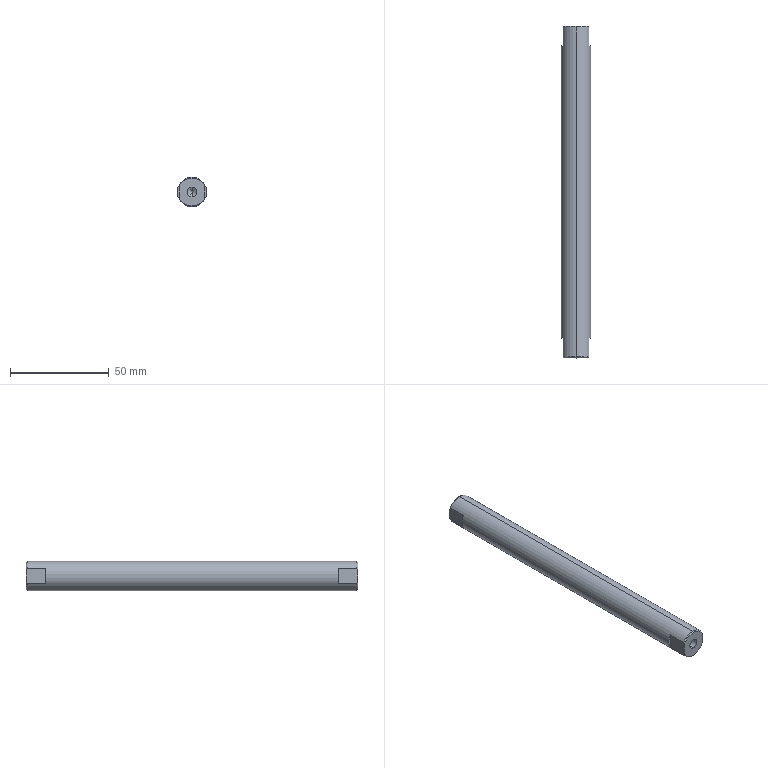Part | SolidWorks | features Chamfer 1, Extrusion 1, HoleWzd 1, ICE 1, MirrorPattern 1 | 1 solid | 26 faces | box 15 x 168 x 15 mm | volume 28790 mm3 | cone 10 | plane 10 | cylinder 6 | commonest cylinder face diameters 5 x4 15 x2
STEP:
#1=CARTESIAN_POINT('',(0.,-67.,2.5));
#2=VERTEX_POINT('',#1);
#3=CARTESIAN_POINT('',(0.,-67.,-2.5));
#4=VERTEX_POINT('',#3);
#5=CARTESIAN_POINT('',(0.,-67.,0.));
#6=DIRECTION('',(0.,-1.,0.));
#7=DIRECTION('',(0.,0.,-1.));
#8=AXIS2_PLACEMENT_3D('',#5,#6,#7);
#9=CIRCLE('',#8,2.5);
#10=EDGE_CURVE('',#2,#4,#9,.T.);
#11=ORIENTED_EDGE('',*,*,#10,.F.);
#12=CARTESIAN_POINT('',(0.,-84.,2.5));
#13=VERTEX_POINT('',#12);
#14=CARTESIAN_POINT('',(0.,-84.,2.5));
#15=DIRECTION('',(0.,-1.,0.));
#16=VECTOR('',#15,1000.);
#17=LINE('',#14,#16);
#18=EDGE_CURVE('',#2,#13,#17,.T.);
#19=ORIENTED_EDGE('',*,*,#18,.T.);
#20=CARTESIAN_POINT('',(0.,-84.,-2.5));
#21=VERTEX_POINT('',#20);
#22=CARTESIAN_POINT('',(0.,-84.,0.));
#23=DIRECTION('',(0.,-1.,0.));
#24=DIRECTION('',(0.,0.,-1.));
#25=AXIS2_PLACEMENT_3D('',#22,#23,#24);
#26=CIRCLE('',#25,2.5);
#27=EDGE_CURVE('',#13,#21,#26,.T.);
#28=ORIENTED_EDGE('',*,*,#27,.T.);
#29=CARTESIAN_POINT('',(0.,-84.,-2.5));
#30=DIRECTION('',(0.,-1.,0.));
#31=VECTOR('',#30,1000.);
#32=LINE('',#29,#31);
#33=EDGE_CURVE('',#4,#21,#32,.T.);
#34=ORIENTED_EDGE('',*,*,#33,.F.);
#35=EDGE_LOOP('',(#11,#19,#28,#34));
#36=FACE_OUTER_BOUND('',#35,.T.);
#37=CARTESIAN_POINT('',(0.,-84.,0.));
#38=DIRECTION('',(0.,-1.,0.));
#39=DIRECTION('',(0.,0.,-1.));
#40=AXIS2_PLACEMENT_3D('',#37,#38,#39);
#41=CYLINDRICAL_SURFACE('',#40,2.5);
#42=ADVANCED_FACE('',(#36),#41,.F.);
#43=CARTESIAN_POINT('',(0.,-65.498,0.));
#44=VERTEX_POINT('',#43);
#45=CARTESIAN_POINT('',(0.,-67.,-2.5));
#46=DIRECTION('',(0.,-0.515,-0.8572));
#47=VECTOR('',#46,1000.);
#48=LINE('',#45,#47);
#49=EDGE_CURVE('',#44,#4,#48,.T.);
#50=ORIENTED_EDGE('',*,*,#49,.F.);
#51=CARTESIAN_POINT('',(0.,-67.,2.5));
#52=DIRECTION('',(0.,-0.515,0.8572));
#53=VECTOR('',#52,1000.);
#54=LINE('',#51,#53);
#55=EDGE_CURVE('',#44,#2,#54,.T.);
#56=ORIENTED_EDGE('',*,*,#55,.T.);
#57=ORIENTED_EDGE('',*,*,#10,.T.);
#58=EDGE_LOOP('',(#50,#56,#57));
#59=FACE_OUTER_BOUND('',#58,.T.);
#60=CARTESIAN_POINT('',(0.,-67.,0.));
#61=DIRECTION('',(0.,-1.,0.));
#62=DIRECTION('',(0.,0.,-1.));
#63=AXIS2_PLACEMENT_3D('',#60,#61,#62);
#64=CONICAL_SURFACE('',#63,2.5,1.03);
#65=ADVANCED_FACE('',(#59),#64,.F.);
#66=CARTESIAN_POINT('',(0.,67.,-2.5));
#67=VERTEX_POINT('',#66);
#68=CARTESIAN_POINT('',(0.,67.,2.5));
#69=VERTEX_POINT('',#68);
#70=CARTESIAN_POINT('',(0.,67.,0.));
#71=DIRECTION('',(0.,1.,0.));
#72=DIRECTION('',(0.,0.,1.));
#73=AXIS2_PLACEMENT_3D('',#70,#71,#72);
#74=CIRCLE('',#73,2.5);
#75=EDGE_CURVE('',#67,#69,#74,.T.);
#76=ORIENTED_EDGE('',*,*,#75,.F.);
#77=CARTESIAN_POINT('',(0.,84.,-2.5));
#78=VERTEX_POINT('',#77);
#79=CARTESIAN_POINT('',(0.,84.,-2.5));
#80=DIRECTION('',(0.,1.,0.));
#81=VECTOR('',#80,1000.);
#82=LINE('',#79,#81);
#83=EDGE_CURVE('',#67,#78,#82,.T.);
#84=ORIENTED_EDGE('',*,*,#83,.T.);
#85=CARTESIAN_POINT('',(0.,84.,2.5));
#86=VERTEX_POINT('',#85);
#87=CARTESIAN_POINT('',(0.,84.,0.));
#88=DIRECTION('',(0.,1.,0.));
#89=DIRECTION('',(0.,0.,1.));
#90=AXIS2_PLACEMENT_3D('',#87,#88,#89);
#91=CIRCLE('',#90,2.5);
#92=EDGE_CURVE('',#78,#86,#91,.T.);
#93=ORIENTED_EDGE('',*,*,#92,.T.);
#94=CARTESIAN_POINT('',(0.,84.,2.5));
#95=DIRECTION('',(0.,1.,0.));
#96=VECTOR('',#95,1000.);
#97=LINE('',#94,#96);
#98=EDGE_CURVE('',#69,#86,#97,.T.);
#99=ORIENTED_EDGE('',*,*,#98,.F.);
#100=EDGE_LOOP('',(#76,#84,#93,#99));
#101=FACE_OUTER_BOUND('',#100,.T.);
#102=CARTESIAN_POINT('',(0.,84.,0.));
#103=DIRECTION('',(0.,1.,0.));
#104=DIRECTION('',(0.,0.,1.));
#105=AXIS2_PLACEMENT_3D('',#102,#103,#104);
#106=CYLINDRICAL_SURFACE('',#105,2.5);
#107=ADVANCED_FACE('',(#101),#106,.F.);
#108=CARTESIAN_POINT('',(0.,65.498,0.));
#109=VERTEX_POINT('',#108);
#110=CARTESIAN_POINT('',(0.,67.,2.5));
#111=DIRECTION('',(0.,0.515,0.8572));
#112=VECTOR('',#111,1000.);
#113=LINE('',#110,#112);
#114=EDGE_CURVE('',#109,#69,#113,.T.);
#115=ORIENTED_EDGE('',*,*,#114,.F.);
#116=CARTESIAN_POINT('',(0.,67.,-2.5));
#117=DIRECTION('',(0.,0.515,-0.8572));
#118=VECTOR('',#117,1000.);
#119=LINE('',#116,#118);
#120=EDGE_CURVE('',#109,#67,#119,.T.);
#121=ORIENTED_EDGE('',*,*,#120,.T.);
#122=ORIENTED_EDGE('',*,*,#75,.T.);
#123=EDGE_LOOP('',(#115,#121,#122));
#124=FACE_OUTER_BOUND('',#123,.T.);
#125=CARTESIAN_POINT('',(0.,67.,0.));
#126=DIRECTION('',(0.,1.,0.));
#127=DIRECTION('',(0.,0.,1.));
#128=AXIS2_PLACEMENT_3D('',#125,#126,#127);
#129=CONICAL_SURFACE('',#128,2.5,1.03);
#130=ADVANCED_FACE('',(#124),#129,.F.);
#131=CARTESIAN_POINT('',(0.,-84.,7.));
#132=VERTEX_POINT('',#131);
#133=CARTESIAN_POINT('',(-6.5,-84.,2.598));
#134=VERTEX_POINT('',#133);
#135=CARTESIAN_POINT('',(0.,-84.,0.));
#136=DIRECTION('',(0.,-1.,0.));
#137=DIRECTION('',(0.,0.,1.));
#138=AXIS2_PLACEMENT_3D('',#135,#136,#137);
#139=CIRCLE('',#138,7.);
#140=EDGE_CURVE('',#132,#134,#139,.T.);
#141=ORIENTED_EDGE('',*,*,#140,.F.);
#142=CARTESIAN_POINT('',(0.,-83.5,7.5));
#143=VERTEX_POINT('',#142);
#144=CARTESIAN_POINT('',(0.,-83.5,7.5));
#145=DIRECTION('',(0.,0.7071,0.7071));
#146=VECTOR('',#145,1000.);
#147=LINE('',#144,#146);
#148=EDGE_CURVE('',#132,#143,#147,.T.);
#149=ORIENTED_EDGE('',*,*,#148,.T.);
#150=CARTESIAN_POINT('',(-6.5,-83.5,3.742));
#151=VERTEX_POINT('',#150);
#152=CARTESIAN_POINT('',(0.,-83.5,0.));
#153=DIRECTION('',(0.,1.,0.));
#154=DIRECTION('',(0.,0.,1.));
#155=AXIS2_PLACEMENT_3D('',#152,#153,#154);
#156=CIRCLE('',#155,7.5);
#157=EDGE_CURVE('',#151,#143,#156,.T.);
#158=ORIENTED_EDGE('',*,*,#157,.F.);
#159=CARTESIAN_POINT('',(-6.5,-84.,2.598));
#160=CARTESIAN_POINT('',(-6.5,-83.854,2.991));
#161=CARTESIAN_POINT('',(-6.5,-83.685,3.371));
#162=CARTESIAN_POINT('',(-6.5,-83.5,3.742));
#163=B_SPLINE_CURVE_WITH_KNOTS('',3,(#159,#160,#161,#162),.UNSPECIFIED.,.F.,.F.,(4,4),(0.02116,0.02241),.UNSPECIFIED.);
#164=EDGE_CURVE('',#134,#151,#163,.T.);
#165=ORIENTED_EDGE('',*,*,#164,.F.);
#166=EDGE_LOOP('',(#141,#149,#158,#165));
#167=FACE_OUTER_BOUND('',#166,.T.);
#168=CARTESIAN_POINT('',(0.,-83.5,0.));
#169=DIRECTION('',(0.,1.,0.));
#170=DIRECTION('',(0.,0.,1.));
#171=AXIS2_PLACEMENT_3D('',#168,#169,#170);
#172=CONICAL_SURFACE('',#171,7.5,0.7854);
#173=ADVANCED_FACE('',(#167),#172,.T.);
#174=CARTESIAN_POINT('',(6.5,83.5,3.742));
#175=VERTEX_POINT('',#174);
#176=CARTESIAN_POINT('',(0.,83.5,7.5));
#177=VERTEX_POINT('',#176);
#178=CARTESIAN_POINT('',(0.,83.5,0.));
#179=DIRECTION('',(0.,-1.,0.));
#180=DIRECTION('',(0.,0.,1.));
#181=AXIS2_PLACEMENT_3D('',#178,#179,#180);
#182=CIRCLE('',#181,7.5);
#183=EDGE_CURVE('',#175,#177,#182,.T.);
#184=ORIENTED_EDGE('',*,*,#183,.T.);
#185=CARTESIAN_POINT('',(0.,84.,7.5));
#186=DIRECTION('',(0.,-1.,0.));
#187=VECTOR('',#186,1000.);
#188=LINE('',#185,#187);
#189=EDGE_CURVE('',#177,#143,#188,.T.);
#190=ORIENTED_EDGE('',*,*,#189,.T.);
#191=CARTESIAN_POINT('',(6.5,-83.5,3.742));
#192=VERTEX_POINT('',#191);
#193=CARTESIAN_POINT('',(0.,-83.5,0.));
#194=DIRECTION('',(0.,1.,0.));
#195=DIRECTION('',(0.,0.,1.));
#196=AXIS2_PLACEMENT_3D('',#193,#194,#195);
#197=CIRCLE('',#196,7.5);
#198=EDGE_CURVE('',#143,#192,#197,.T.);
#199=ORIENTED_EDGE('',*,*,#198,.T.);
#200=CARTESIAN_POINT('',(6.5,-74.,3.742));
#201=VERTEX_POINT('',#200);
#202=CARTESIAN_POINT('',(6.5,84.,3.742));
#203=DIRECTION('',(0.,1.,0.));
#204=VECTOR('',#203,1000.);
#205=LINE('',#202,#204);
#206=EDGE_CURVE('',#192,#201,#205,.T.);
#207=ORIENTED_EDGE('',*,*,#206,.T.);
#208=CARTESIAN_POINT('',(6.5,-74.,-3.742));
#209=VERTEX_POINT('',#208);
#210=CARTESIAN_POINT('',(0.,-74.,0.));
#211=DIRECTION('',(0.,1.,0.));
#212=DIRECTION('',(0.,0.,1.));
#213=AXIS2_PLACEMENT_3D('',#210,#211,#212);
#214=CIRCLE('',#213,7.5);
#215=EDGE_CURVE('',#201,#209,#214,.T.);
#216=ORIENTED_EDGE('',*,*,#215,.T.);
#217=CARTESIAN_POINT('',(6.5,-83.5,-3.742));
#218=VERTEX_POINT('',#217);
#219=CARTESIAN_POINT('',(6.5,84.,-3.742));
#220=DIRECTION('',(0.,-1.,0.));
#221=VECTOR('',#220,1000.);
#222=LINE('',#219,#221);
#223=EDGE_CURVE('',#209,#218,#222,.T.);
#224=ORIENTED_EDGE('',*,*,#223,.T.);
#225=CARTESIAN_POINT('',(0.,-83.5,-7.5));
#226=VERTEX_POINT('',#225);
#227=CARTESIAN_POINT('',(0.,-83.5,0.));
#228=DIRECTION('',(0.,1.,0.));
#229=DIRECTION('',(0.,0.,1.));
#230=AXIS2_PLACEMENT_3D('',#227,#228,#229);
#231=CIRCLE('',#230,7.5);
#232=EDGE_CURVE('',#218,#226,#231,.T.);
#233=ORIENTED_EDGE('',*,*,#232,.T.);
#234=CARTESIAN_POINT('',(0.,83.5,-7.5));
#235=VERTEX_POINT('',#234);
#236=CARTESIAN_POINT('',(0.,84.,-7.5));
#237=DIRECTION('',(0.,-1.,0.));
#238=VECTOR('',#237,1000.);
#239=LINE('',#236,#238);
#240=EDGE_CURVE('',#235,#226,#239,.T.);
#241=ORIENTED_EDGE('',*,*,#240,.F.);
#242=CARTESIAN_POINT('',(6.5,83.5,-3.742));
#243=VERTEX_POINT('',#242);
#244=CARTESIAN_POINT('',(0.,83.5,0.));
#245=DIRECTION('',(0.,-1.,0.));
#246=DIRECTION('',(0.,0.,1.));
#247=AXIS2_PLACEMENT_3D('',#244,#245,#246);
#248=CIRCLE('',#247,7.5);
#249=EDGE_CURVE('',#235,#243,#248,.T.);
#250=ORIENTED_EDGE('',*,*,#249,.T.);
#251=CARTESIAN_POINT('',(6.5,74.,-3.742));
#252=VERTEX_POINT('',#251);
#253=CARTESIAN_POINT('',(6.5,84.,-3.742));
#254=DIRECTION('',(0.,-1.,0.));
#255=VECTOR('',#254,1000.);
#256=LINE('',#253,#255);
#257=EDGE_CURVE('',#243,#252,#256,.T.);
#258=ORIENTED_EDGE('',*,*,#257,.T.);
#259=CARTESIAN_POINT('',(6.5,74.,3.742));
#260=VERTEX_POINT('',#259);
#261=CARTESIAN_POINT('',(0.,74.,0.));
#262=DIRECTION('',(0.,-1.,0.));
#263=DIRECTION('',(0.,0.,-1.));
#264=AXIS2_PLACEMENT_3D('',#261,#262,#263);
#265=CIRCLE('',#264,7.5);
#266=EDGE_CURVE('',#252,#260,#265,.T.);
#267=ORIENTED_EDGE('',*,*,#266,.T.);
#268=CARTESIAN_POINT('',(6.5,84.,3.742));
#269=DIRECTION('',(0.,1.,0.));
#270=VECTOR('',#269,1000.);
#271=LINE('',#268,#270);
#272=EDGE_CURVE('',#260,#175,#271,.T.);
#273=ORIENTED_EDGE('',*,*,#272,.T.);
#274=EDGE_LOOP('',(#184,#190,#199,#207,#216,#224,#233,#241,#250,#258,#267,#273));
#275=FACE_OUTER_BOUND('',#274,.T.);
#276=CARTESIAN_POINT('',(0.,84.,0.));
#277=DIRECTION('',(0.,-1.,0.));
#278=DIRECTION('',(0.,0.,-1.));
#279=AXIS2_PLACEMENT_3D('',#276,#277,#278);
#280=CYLINDRICAL_SURFACE('',#279,7.5);
#281=ADVANCED_FACE('',(#275),#280,.T.);
#282=CARTESIAN_POINT('',(0.,84.,-7.));
#283=VERTEX_POINT('',#282);
#284=CARTESIAN_POINT('',(-6.5,84.,-2.598));
#285=VERTEX_POINT('',#284);
#286=CARTESIAN_POINT('',(0.,84.,0.));
#287=DIRECTION('',(0.,1.,0.));
#288=DIRECTION('',(0.,0.,1.));
#289=AXIS2_PLACEMENT_3D('',#286,#287,#288);
#290=CIRCLE('',#289,7.);
#291=EDGE_CURVE('',#283,#285,#290,.T.);
#292=ORIENTED_EDGE('',*,*,#291,.F.);
#293=CARTESIAN_POINT('',(0.,84.,-7.));
#294=DIRECTION('',(0.,-0.7071,-0.7071));
#295=VECTOR('',#294,1000.);
#296=LINE('',#293,#295);
#297=EDGE_CURVE('',#283,#235,#296,.T.);
#298=ORIENTED_EDGE('',*,*,#297,.T.);
#299=CARTESIAN_POINT('',(-6.5,83.5,-3.742));
#300=VERTEX_POINT('',#299);
#301=CARTESIAN_POINT('',(0.,83.5,0.));
#302=DIRECTION('',(0.,-1.,0.));
#303=DIRECTION('',(0.,0.,1.));
#304=AXIS2_PLACEMENT_3D('',#301,#302,#303);
#305=CIRCLE('',#304,7.5);
#306=EDGE_CURVE('',#300,#235,#305,.T.);
#307=ORIENTED_EDGE('',*,*,#306,.F.);
#308=CARTESIAN_POINT('',(-6.5,84.,-2.598));
#309=CARTESIAN_POINT('',(-6.5,83.854,-2.991));
#310=CARTESIAN_POINT('',(-6.5,83.685,-3.371));
#311=CARTESIAN_POINT('',(-6.5,83.5,-3.742));
#312=B_SPLINE_CURVE_WITH_KNOTS('',3,(#308,#309,#310,#311),.UNSPECIFIED.,.F.,.F.,(4,4),(0.02116,0.02241),.UNSPECIFIED.);
#313=EDGE_CURVE('',#285,#300,#312,.T.);
#314=ORIENTED_EDGE('',*,*,#313,.F.);
#315=EDGE_LOOP('',(#292,#298,#307,#314));
#316=FACE_OUTER_BOUND('',#315,.T.);
#317=CARTESIAN_POINT('',(0.,84.,0.));
#318=DIRECTION('',(0.,-1.,0.));
#319=DIRECTION('',(0.,0.,-1.));
#320=AXIS2_PLACEMENT_3D('',#317,#318,#319);
#321=CONICAL_SURFACE('',#320,7.,0.7854);
#322=ADVANCED_FACE('',(#316),#321,.T.);
#323=CARTESIAN_POINT('',(-6.5,-83.5,-3.742));
#324=VERTEX_POINT('',#323);
#325=CARTESIAN_POINT('',(-6.5,-84.,-2.598));
#326=VERTEX_POINT('',#325);
#327=CARTESIAN_POINT('',(-6.5,-83.5,-3.742));
#328=CARTESIAN_POINT('',(-6.5,-83.686,-3.369));
#329=CARTESIAN_POINT('',(-6.5,-83.855,-2.989));
#330=CARTESIAN_POINT('',(-6.5,-84.,-2.598));
#331=B_SPLINE_CURVE_WITH_KNOTS('',3,(#327,#328,#329,#330),.UNSPECIFIED.,.F.,.F.,(4,4),(0.01459,0.01584),.UNSPECIFIED.);
#332=EDGE_CURVE('',#324,#326,#331,.T.);
#333=ORIENTED_EDGE('',*,*,#332,.F.);
#334=CARTESIAN_POINT('',(0.,-83.5,0.));
#335=DIRECTION('',(0.,1.,0.));
#336=DIRECTION('',(0.,0.,1.));
#337=AXIS2_PLACEMENT_3D('',#334,#335,#336);
#338=CIRCLE('',#337,7.5);
#339=EDGE_CURVE('',#226,#324,#338,.T.);
#340=ORIENTED_EDGE('',*,*,#339,.F.);
#341=ORIENTED_EDGE('',*,*,#232,.F.);
#342=CARTESIAN_POINT('',(6.5,-84.,-2.598));
#343=VERTEX_POINT('',#342);
#344=CARTESIAN_POINT('',(6.5,-84.,-2.598));
#345=CARTESIAN_POINT('',(6.5,-83.854,-2.991));
#346=CARTESIAN_POINT('',(6.5,-83.685,-3.371));
#347=CARTESIAN_POINT('',(6.5,-83.5,-3.742));
#348=B_SPLINE_CURVE_WITH_KNOTS('',3,(#344,#345,#346,#347),.UNSPECIFIED.,.F.,.F.,(4,4),(0.02116,0.02241),.UNSPECIFIED.);
#349=EDGE_CURVE('',#343,#218,#348,.T.);
#350=ORIENTED_EDGE('',*,*,#349,.F.);
#351=CARTESIAN_POINT('',(0.,-84.,0.));
#352=DIRECTION('',(0.,-1.,0.));
#353=DIRECTION('',(0.,0.,1.));
#354=AXIS2_PLACEMENT_3D('',#351,#352,#353);
#355=CIRCLE('',#354,7.);
#356=EDGE_CURVE('',#326,#343,#355,.T.);
#357=ORIENTED_EDGE('',*,*,#356,.F.);
#358=EDGE_LOOP('',(#333,#340,#341,#350,#357));
#359=FACE_OUTER_BOUND('',#358,.T.);
#360=CARTESIAN_POINT('',(0.,-83.5,0.));
#361=DIRECTION('',(0.,1.,0.));
#362=DIRECTION('',(0.,0.,1.));
#363=AXIS2_PLACEMENT_3D('',#360,#361,#362);
#364=CONICAL_SURFACE('',#363,7.5,0.7854);
#365=ADVANCED_FACE('',(#359),#364,.T.);
#366=ORIENTED_EDGE('',*,*,#297,.F.);
#367=CARTESIAN_POINT('',(6.5,84.,-2.598));
#368=VERTEX_POINT('',#367);
#369=CARTESIAN_POINT('',(0.,84.,0.));
#370=DIRECTION('',(0.,1.,0.));
#371=DIRECTION('',(0.,0.,1.));
#372=AXIS2_PLACEMENT_3D('',#369,#370,#371);
#373=CIRCLE('',#372,7.);
#374=EDGE_CURVE('',#368,#283,#373,.T.);
#375=ORIENTED_EDGE('',*,*,#374,.F.);
#376=CARTESIAN_POINT('',(6.5,83.5,-3.742));
#377=CARTESIAN_POINT('',(6.5,83.686,-3.369));
#378=CARTESIAN_POINT('',(6.5,83.855,-2.989));
#379=CARTESIAN_POINT('',(6.5,84.,-2.598));
#380=B_SPLINE_CURVE_WITH_KNOTS('',3,(#376,#377,#378,#379),.UNSPECIFIED.,.F.,.F.,(4,4),(0.01459,0.01584),.UNSPECIFIED.);
#381=EDGE_CURVE('',#243,#368,#380,.T.);
#382=ORIENTED_EDGE('',*,*,#381,.F.);
#383=ORIENTED_EDGE('',*,*,#249,.F.);
#384=EDGE_LOOP('',(#366,#375,#382,#383));
#385=FACE_OUTER_BOUND('',#384,.T.);
#386=CARTESIAN_POINT('',(0.,84.,0.));
#387=DIRECTION('',(0.,-1.,0.));
#388=DIRECTION('',(0.,0.,-1.));
#389=AXIS2_PLACEMENT_3D('',#386,#387,#388);
#390=CONICAL_SURFACE('',#389,7.,0.7854);
#391=ADVANCED_FACE('',(#385),#390,.T.);
#392=ORIENTED_EDGE('',*,*,#189,.F.);
#393=CARTESIAN_POINT('',(-6.5,83.5,3.742));
#394=VERTEX_POINT('',#393);
#395=CARTESIAN_POINT('',(0.,83.5,0.));
#396=DIRECTION('',(0.,-1.,0.));
#397=DIRECTION('',(0.,0.,1.));
#398=AXIS2_PLACEMENT_3D('',#395,#396,#397);
#399=CIRCLE('',#398,7.5);
#400=EDGE_CURVE('',#177,#394,#399,.T.);
#401=ORIENTED_EDGE('',*,*,#400,.T.);
#402=CARTESIAN_POINT('',(-6.5,74.,3.742));
#403=VERTEX_POINT('',#402);
#404=CARTESIAN_POINT('',(-6.5,84.,3.742));
#405=DIRECTION('',(0.,-1.,0.));
#406=VECTOR('',#405,1000.);
#407=LINE('',#404,#406);
#408=EDGE_CURVE('',#394,#403,#407,.T.);
#409=ORIENTED_EDGE('',*,*,#408,.T.);
#410=CARTESIAN_POINT('',(-6.5,74.,-3.742));
#411=VERTEX_POINT('',#410);
#412=CARTESIAN_POINT('',(0.,74.,0.));
#413=DIRECTION('',(0.,-1.,0.));
#414=DIRECTION('',(0.,0.,-1.));
#415=AXIS2_PLACEMENT_3D('',#412,#413,#414);
#416=CIRCLE('',#415,7.5);
#417=EDGE_CURVE('',#403,#411,#416,.T.);
#418=ORIENTED_EDGE('',*,*,#417,.T.);
#419=CARTESIAN_POINT('',(-6.5,84.,-3.742));
#420=DIRECTION('',(0.,1.,0.));
#421=VECTOR('',#420,1000.);
#422=LINE('',#419,#421);
#423=EDGE_CURVE('',#411,#300,#422,.T.);
#424=ORIENTED_EDGE('',*,*,#423,.T.);
#425=ORIENTED_EDGE('',*,*,#306,.T.);
#426=ORIENTED_EDGE('',*,*,#240,.T.);
#427=ORIENTED_EDGE('',*,*,#339,.T.);
#428=CARTESIAN_POINT('',(-6.5,-74.,-3.742));
#429=VERTEX_POINT('',#428);
#430=CARTESIAN_POINT('',(-6.5,84.,-3.742));
#431=DIRECTION('',(0.,1.,0.));
#432=VECTOR('',#431,1000.);
#433=LINE('',#430,#432);
#434=EDGE_CURVE('',#324,#429,#433,.T.);
#435=ORIENTED_EDGE('',*,*,#434,.T.);
#436=CARTESIAN_POINT('',(-6.5,-74.,3.742));
#437=VERTEX_POINT('',#436);
#438=CARTESIAN_POINT('',(0.,-74.,0.));
#439=DIRECTION('',(0.,1.,0.));
#440=DIRECTION('',(0.,0.,1.));
#441=AXIS2_PLACEMENT_3D('',#438,#439,#440);
#442=CIRCLE('',#441,7.5);
#443=EDGE_CURVE('',#429,#437,#442,.T.);
#444=ORIENTED_EDGE('',*,*,#443,.T.);
#445=CARTESIAN_POINT('',(-6.5,84.,3.742));
#446=DIRECTION('',(0.,-1.,0.));
#447=VECTOR('',#446,1000.);
#448=LINE('',#445,#447);
#449=EDGE_CURVE('',#437,#151,#448,.T.);
#450=ORIENTED_EDGE('',*,*,#449,.T.);
#451=ORIENTED_EDGE('',*,*,#157,.T.);
#452=EDGE_LOOP('',(#392,#401,#409,#418,#424,#425,#426,#427,#435,#444,#450,#451));
#453=FACE_OUTER_BOUND('',#452,.T.);
#454=CARTESIAN_POINT('',(0.,84.,0.));
#455=DIRECTION('',(0.,-1.,0.));
#456=DIRECTION('',(0.,0.,-1.));
#457=AXIS2_PLACEMENT_3D('',#454,#455,#456);
#458=CYLINDRICAL_SURFACE('',#457,7.5);
#459=ADVANCED_FACE('',(#453),#458,.T.);
#460=CARTESIAN_POINT('',(6.5,84.,2.598));
#461=VERTEX_POINT('',#460);
#462=CARTESIAN_POINT('',(6.5,84.,-10.));
#463=DIRECTION('',(0.,0.,1.));
#464=VECTOR('',#463,1000.);
#465=LINE('',#462,#464);
#466=EDGE_CURVE('',#368,#461,#465,.T.);
#467=ORIENTED_EDGE('',*,*,#466,.F.);
#468=ORIENTED_EDGE('',*,*,#374,.T.);
#469=ORIENTED_EDGE('',*,*,#291,.T.);
#470=CARTESIAN_POINT('',(-6.5,84.,2.598));
#471=VERTEX_POINT('',#470);
#472=CARTESIAN_POINT('',(-6.5,84.,-10.));
#473=DIRECTION('',(0.,0.,1.));
#474=VECTOR('',#473,1000.);
#475=LINE('',#472,#474);
#476=EDGE_CURVE('',#285,#471,#475,.T.);
#477=ORIENTED_EDGE('',*,*,#476,.T.);
#478=CARTESIAN_POINT('',(0.,84.,0.));
#479=DIRECTION('',(0.,1.,0.));
#480=DIRECTION('',(0.,0.,1.));
#481=AXIS2_PLACEMENT_3D('',#478,#479,#480);
#482=CIRCLE('',#481,7.);
#483=EDGE_CURVE('',#471,#461,#482,.T.);
#484=ORIENTED_EDGE('',*,*,#483,.T.);
#485=EDGE_LOOP('',(#467,#468,#469,#477,#484));
#486=FACE_OUTER_BOUND('',#485,.T.);
#487=CARTESIAN_POINT('',(0.,84.,0.));
#488=DIRECTION('',(0.,1.,0.));
#489=DIRECTION('',(0.,0.,1.));
#490=AXIS2_PLACEMENT_3D('',#487,#488,#489);
#491=CIRCLE('',#490,2.5);
#492=EDGE_CURVE('',#86,#78,#491,.T.);
#493=ORIENTED_EDGE('',*,*,#492,.F.);
#494=ORIENTED_EDGE('',*,*,#92,.F.);
#495=EDGE_LOOP('',(#493,#494));
#496=FACE_BOUND('',#495,.T.);
#497=CARTESIAN_POINT('',(0.,84.,0.));
#498=DIRECTION('',(0.,1.,0.));
#499=DIRECTION('',(0.,0.,1.));
#500=AXIS2_PLACEMENT_3D('',#497,#498,#499);
#501=PLANE('',#500);
#502=ADVANCED_FACE('',(#486,#496),#501,.T.);
#503=CARTESIAN_POINT('',(0.,-84.,0.));
#504=DIRECTION('',(0.,-1.,0.));
#505=DIRECTION('',(0.,0.,-1.));
#506=AXIS2_PLACEMENT_3D('',#503,#504,#505);
#507=CIRCLE('',#506,2.5);
#508=EDGE_CURVE('',#21,#13,#507,.T.);
#509=ORIENTED_EDGE('',*,*,#508,.F.);
#510=ORIENTED_EDGE('',*,*,#27,.F.);
#511=EDGE_LOOP('',(#509,#510));
#512=FACE_BOUND('',#511,.T.);
#513=CARTESIAN_POINT('',(6.5,-84.,2.598));
#514=VERTEX_POINT('',#513);
#515=CARTESIAN_POINT('',(0.,-84.,0.));
#516=DIRECTION('',(0.,-1.,0.));
#517=DIRECTION('',(0.,0.,1.));
#518=AXIS2_PLACEMENT_3D('',#515,#516,#517);
#519=CIRCLE('',#518,7.);
#520=EDGE_CURVE('',#514,#132,#519,.T.);
#521=ORIENTED_EDGE('',*,*,#520,.T.);
#522=ORIENTED_EDGE('',*,*,#140,.T.);
#523=CARTESIAN_POINT('',(-6.5,-84.,-10.));
#524=DIRECTION('',(0.,0.,1.));
#525=VECTOR('',#524,1000.);
#526=LINE('',#523,#525);
#527=EDGE_CURVE('',#326,#134,#526,.T.);
#528=ORIENTED_EDGE('',*,*,#527,.F.);
#529=ORIENTED_EDGE('',*,*,#356,.T.);
#530=CARTESIAN_POINT('',(6.5,-84.,-10.));
#531=DIRECTION('',(0.,0.,1.));
#532=VECTOR('',#531,1000.);
#533=LINE('',#530,#532);
#534=EDGE_CURVE('',#343,#514,#533,.T.);
#535=ORIENTED_EDGE('',*,*,#534,.T.);
#536=EDGE_LOOP('',(#521,#522,#528,#529,#535));
#537=FACE_OUTER_BOUND('',#536,.T.);
#538=CARTESIAN_POINT('',(0.,-84.,0.));
#539=DIRECTION('',(0.,1.,0.));
#540=DIRECTION('',(0.,0.,1.));
#541=AXIS2_PLACEMENT_3D('',#538,#539,#540);
#542=PLANE('',#541);
#543=ADVANCED_FACE('',(#512,#537),#542,.F.);
#544=ORIENTED_EDGE('',*,*,#148,.F.);
#545=ORIENTED_EDGE('',*,*,#520,.F.);
#546=CARTESIAN_POINT('',(6.5,-83.5,3.742));
#547=CARTESIAN_POINT('',(6.5,-83.686,3.369));
#548=CARTESIAN_POINT('',(6.5,-83.855,2.989));
#549=CARTESIAN_POINT('',(6.5,-84.,2.598));
#550=B_SPLINE_CURVE_WITH_KNOTS('',3,(#546,#547,#548,#549),.UNSPECIFIED.,.F.,.F.,(4,4),(0.01459,0.01584),.UNSPECIFIED.);
#551=EDGE_CURVE('',#192,#514,#550,.T.);
#552=ORIENTED_EDGE('',*,*,#551,.F.);
#553=ORIENTED_EDGE('',*,*,#198,.F.);
#554=EDGE_LOOP('',(#544,#545,#552,#553));
#555=FACE_OUTER_BOUND('',#554,.T.);
#556=CARTESIAN_POINT('',(0.,-83.5,0.));
#557=DIRECTION('',(0.,1.,0.));
#558=DIRECTION('',(0.,0.,1.));
#559=AXIS2_PLACEMENT_3D('',#556,#557,#558);
#560=CONICAL_SURFACE('',#559,7.5,0.7854);
#561=ADVANCED_FACE('',(#555),#560,.T.);
#562=CARTESIAN_POINT('',(6.5,84.,2.598));
#563=CARTESIAN_POINT('',(6.5,83.854,2.991));
#564=CARTESIAN_POINT('',(6.5,83.685,3.371));
#565=CARTESIAN_POINT('',(6.5,83.5,3.742));
#566=B_SPLINE_CURVE_WITH_KNOTS('',3,(#562,#563,#564,#565),.UNSPECIFIED.,.F.,.F.,(4,4),(0.02116,0.02241),.UNSPECIFIED.);
#567=EDGE_CURVE('',#461,#175,#566,.T.);
#568=ORIENTED_EDGE('',*,*,#567,.F.);
#569=ORIENTED_EDGE('',*,*,#483,.F.);
#570=CARTESIAN_POINT('',(-6.5,83.5,3.742));
#571=CARTESIAN_POINT('',(-6.5,83.686,3.369));
#572=CARTESIAN_POINT('',(-6.5,83.855,2.989));
#573=CARTESIAN_POINT('',(-6.5,84.,2.598));
#574=B_SPLINE_CURVE_WITH_KNOTS('',3,(#570,#571,#572,#573),.UNSPECIFIED.,.F.,.F.,(4,4),(0.01459,0.01584),.UNSPECIFIED.);
#575=EDGE_CURVE('',#394,#471,#574,.T.);
#576=ORIENTED_EDGE('',*,*,#575,.F.);
#577=ORIENTED_EDGE('',*,*,#400,.F.);
#578=ORIENTED_EDGE('',*,*,#183,.F.);
#579=EDGE_LOOP('',(#568,#569,#576,#577,#578));
#580=FACE_OUTER_BOUND('',#579,.T.);
#581=CARTESIAN_POINT('',(0.,84.,0.));
#582=DIRECTION('',(0.,-1.,0.));
#583=DIRECTION('',(0.,0.,-1.));
#584=AXIS2_PLACEMENT_3D('',#581,#582,#583);
#585=CONICAL_SURFACE('',#584,7.,0.7854);
#586=ADVANCED_FACE('',(#580),#585,.T.);
#587=ORIENTED_EDGE('',*,*,#120,.F.);
#588=ORIENTED_EDGE('',*,*,#114,.T.);
#589=CARTESIAN_POINT('',(0.,67.,0.));
#590=DIRECTION('',(0.,1.,0.));
#591=DIRECTION('',(0.,0.,1.));
#592=AXIS2_PLACEMENT_3D('',#589,#590,#591);
#593=CIRCLE('',#592,2.5);
#594=EDGE_CURVE('',#69,#67,#593,.T.);
#595=ORIENTED_EDGE('',*,*,#594,.T.);
#596=EDGE_LOOP('',(#587,#588,#595));
#597=FACE_OUTER_BOUND('',#596,.T.);
#598=CARTESIAN_POINT('',(0.,67.,0.));
#599=DIRECTION('',(0.,1.,0.));
#600=DIRECTION('',(0.,0.,1.));
#601=AXIS2_PLACEMENT_3D('',#598,#599,#600);
#602=CONICAL_SURFACE('',#601,2.5,1.03);
#603=ADVANCED_FACE('',(#597),#602,.F.);
#604=ORIENTED_EDGE('',*,*,#83,.F.);
#605=ORIENTED_EDGE('',*,*,#594,.F.);
#606=ORIENTED_EDGE('',*,*,#98,.T.);
#607=ORIENTED_EDGE('',*,*,#492,.T.);
#608=EDGE_LOOP('',(#604,#605,#606,#607));
#609=FACE_OUTER_BOUND('',#608,.T.);
#610=CARTESIAN_POINT('',(0.,84.,0.));
#611=DIRECTION('',(0.,1.,0.));
#612=DIRECTION('',(0.,0.,1.));
#613=AXIS2_PLACEMENT_3D('',#610,#611,#612);
#614=CYLINDRICAL_SURFACE('',#613,2.5);
#615=ADVANCED_FACE('',(#609),#614,.F.);
#616=ORIENTED_EDGE('',*,*,#55,.F.);
#617=ORIENTED_EDGE('',*,*,#49,.T.);
#618=CARTESIAN_POINT('',(0.,-67.,0.));
#619=DIRECTION('',(0.,-1.,0.));
#620=DIRECTION('',(0.,0.,-1.));
#621=AXIS2_PLACEMENT_3D('',#618,#619,#620);
#622=CIRCLE('',#621,2.5);
#623=EDGE_CURVE('',#4,#2,#622,.T.);
#624=ORIENTED_EDGE('',*,*,#623,.T.);
#625=EDGE_LOOP('',(#616,#617,#624));
#626=FACE_OUTER_BOUND('',#625,.T.);
#627=CARTESIAN_POINT('',(0.,-67.,0.));
#628=DIRECTION('',(0.,-1.,0.));
#629=DIRECTION('',(0.,0.,-1.));
#630=AXIS2_PLACEMENT_3D('',#627,#628,#629);
#631=CONICAL_SURFACE('',#630,2.5,1.03);
#632=ADVANCED_FACE('',(#626),#631,.F.);
#633=ORIENTED_EDGE('',*,*,#18,.F.);
#634=ORIENTED_EDGE('',*,*,#623,.F.);
#635=ORIENTED_EDGE('',*,*,#33,.T.);
#636=ORIENTED_EDGE('',*,*,#508,.T.);
#637=EDGE_LOOP('',(#633,#634,#635,#636));
#638=FACE_OUTER_BOUND('',#637,.T.);
#639=CARTESIAN_POINT('',(0.,-84.,0.));
#640=DIRECTION('',(0.,-1.,0.));
#641=DIRECTION('',(0.,0.,-1.));
#642=AXIS2_PLACEMENT_3D('',#639,#640,#641);
#643=CYLINDRICAL_SURFACE('',#642,2.5);
#644=ADVANCED_FACE('',(#638),#643,.F.);
#645=CARTESIAN_POINT('',(-6.5,74.,-10.));
#646=DIRECTION('',(0.,0.,1.));
#647=VECTOR('',#646,1000.);
#648=LINE('',#645,#647);
#649=EDGE_CURVE('',#411,#403,#648,.T.);
#650=ORIENTED_EDGE('',*,*,#649,.F.);
#651=ORIENTED_EDGE('',*,*,#417,.F.);
#652=EDGE_LOOP('',(#650,#651));
#653=FACE_OUTER_BOUND('',#652,.T.);
#654=CARTESIAN_POINT('',(-7.5,74.,-10.));
#655=DIRECTION('',(0.,-1.,0.));
#656=DIRECTION('',(0.,0.,-1.));
#657=AXIS2_PLACEMENT_3D('',#654,#655,#656);
#658=PLANE('',#657);
#659=ADVANCED_FACE('',(#653),#658,.F.);
#660=ORIENTED_EDGE('',*,*,#575,.T.);
#661=ORIENTED_EDGE('',*,*,#476,.F.);
#662=ORIENTED_EDGE('',*,*,#313,.T.);
#663=ORIENTED_EDGE('',*,*,#423,.F.);
#664=ORIENTED_EDGE('',*,*,#649,.T.);
#665=ORIENTED_EDGE('',*,*,#408,.F.);
#666=EDGE_LOOP('',(#660,#661,#662,#663,#664,#665));
#667=FACE_OUTER_BOUND('',#666,.T.);
#668=CARTESIAN_POINT('',(-6.5,74.,-10.));
#669=DIRECTION('',(1.,0.,0.));
#670=DIRECTION('',(0.,0.,-1.));
#671=AXIS2_PLACEMENT_3D('',#668,#669,#670);
#672=PLANE('',#671);
#673=ADVANCED_FACE('',(#667),#672,.F.);
#674=CARTESIAN_POINT('',(6.5,74.,-10.));
#675=DIRECTION('',(0.,0.,1.));
#676=VECTOR('',#675,1000.);
#677=LINE('',#674,#676);
#678=EDGE_CURVE('',#252,#260,#677,.T.);
#679=ORIENTED_EDGE('',*,*,#678,.T.);
#680=ORIENTED_EDGE('',*,*,#266,.F.);
#681=EDGE_LOOP('',(#679,#680));
#682=FACE_OUTER_BOUND('',#681,.T.);
#683=CARTESIAN_POINT('',(7.5,74.,-10.));
#684=DIRECTION('',(0.,-1.,0.));
#685=DIRECTION('',(0.,0.,-1.));
#686=AXIS2_PLACEMENT_3D('',#683,#684,#685);
#687=PLANE('',#686);
#688=ADVANCED_FACE('',(#682),#687,.F.);
#689=ORIENTED_EDGE('',*,*,#381,.T.);
#690=ORIENTED_EDGE('',*,*,#466,.T.);
#691=ORIENTED_EDGE('',*,*,#567,.T.);
#692=ORIENTED_EDGE('',*,*,#272,.F.);
#693=ORIENTED_EDGE('',*,*,#678,.F.);
#694=ORIENTED_EDGE('',*,*,#257,.F.);
#695=EDGE_LOOP('',(#689,#690,#691,#692,#693,#694));
#696=FACE_OUTER_BOUND('',#695,.T.);
#697=CARTESIAN_POINT('',(6.5,74.,-10.));
#698=DIRECTION('',(-1.,0.,0.));
#699=DIRECTION('',(0.,-1.,0.));
#700=AXIS2_PLACEMENT_3D('',#697,#698,#699);
#701=PLANE('',#700);
#702=ADVANCED_FACE('',(#696),#701,.F.);
#703=CARTESIAN_POINT('',(6.5,-74.,-10.));
#704=DIRECTION('',(0.,0.,1.));
#705=VECTOR('',#704,1000.);
#706=LINE('',#703,#705);
#707=EDGE_CURVE('',#209,#201,#706,.T.);
#708=ORIENTED_EDGE('',*,*,#707,.F.);
#709=ORIENTED_EDGE('',*,*,#215,.F.);
#710=EDGE_LOOP('',(#708,#709));
#711=FACE_OUTER_BOUND('',#710,.T.);
#712=CARTESIAN_POINT('',(7.5,-74.,-10.));
#713=DIRECTION('',(0.,1.,0.));
#714=DIRECTION('',(0.,0.,1.));
#715=AXIS2_PLACEMENT_3D('',#712,#713,#714);
#716=PLANE('',#715);
#717=ADVANCED_FACE('',(#711),#716,.F.);
#718=ORIENTED_EDGE('',*,*,#551,.T.);
#719=ORIENTED_EDGE('',*,*,#534,.F.);
#720=ORIENTED_EDGE('',*,*,#349,.T.);
#721=ORIENTED_EDGE('',*,*,#223,.F.);
#722=ORIENTED_EDGE('',*,*,#707,.T.);
#723=ORIENTED_EDGE('',*,*,#206,.F.);
#724=EDGE_LOOP('',(#718,#719,#720,#721,#722,#723));
#725=FACE_OUTER_BOUND('',#724,.T.);
#726=CARTESIAN_POINT('',(6.5,-74.,-10.));
#727=DIRECTION('',(-1.,0.,0.));
#728=DIRECTION('',(0.,-1.,0.));
#729=AXIS2_PLACEMENT_3D('',#726,#727,#728);
#730=PLANE('',#729);
#731=ADVANCED_FACE('',(#725),#730,.F.);
#732=CARTESIAN_POINT('',(-6.5,-74.,-10.));
#733=DIRECTION('',(0.,0.,1.));
#734=VECTOR('',#733,1000.);
#735=LINE('',#732,#734);
#736=EDGE_CURVE('',#429,#437,#735,.T.);
#737=ORIENTED_EDGE('',*,*,#736,.T.);
#738=ORIENTED_EDGE('',*,*,#443,.F.);
#739=EDGE_LOOP('',(#737,#738));
#740=FACE_OUTER_BOUND('',#739,.T.);
#741=CARTESIAN_POINT('',(-7.5,-74.,-10.));
#742=DIRECTION('',(0.,1.,0.));
#743=DIRECTION('',(0.,0.,1.));
#744=AXIS2_PLACEMENT_3D('',#741,#742,#743);
#745=PLANE('',#744);
#746=ADVANCED_FACE('',(#740),#745,.F.);
#747=ORIENTED_EDGE('',*,*,#332,.T.);
#748=ORIENTED_EDGE('',*,*,#527,.T.);
#749=ORIENTED_EDGE('',*,*,#164,.T.);
#750=ORIENTED_EDGE('',*,*,#449,.F.);
#751=ORIENTED_EDGE('',*,*,#736,.F.);
#752=ORIENTED_EDGE('',*,*,#434,.F.);
#753=EDGE_LOOP('',(#747,#748,#749,#750,#751,#752));
#754=FACE_OUTER_BOUND('',#753,.T.);
#755=CARTESIAN_POINT('',(-6.5,-74.,-10.));
#756=DIRECTION('',(1.,0.,0.));
#757=DIRECTION('',(0.,1.,0.));
#758=AXIS2_PLACEMENT_3D('',#755,#756,#757);
#759=PLANE('',#758);
#760=ADVANCED_FACE('',(#754),#759,.F.);
#761=CLOSED_SHELL('',(#42,#65,#107,#130,#173,#281,#322,#365,#391,#459,#502,#543,#561,#586,#603,#615,#632,#644,#659,#673,#688,#702,#717,#731,#746,#760));
#762=MANIFOLD_SOLID_BREP('',#761);
#763=CARTESIAN_POINT('',(0.,0.,0.));
#764=DIRECTION('',(0.,0.,1.));
#765=DIRECTION('',(1.,0.,0.));
#766=AXIS2_PLACEMENT_3D('',#763,#764,#765);
#767=(LENGTH_UNIT()NAMED_UNIT(*)SI_UNIT(.MILLI.,.METRE.));
#768=UNCERTAINTY_MEASURE_WITH_UNIT(LENGTH_MEASURE(0.00001),#767,'','');
#769=(NAMED_UNIT(*)PLANE_ANGLE_UNIT()SI_UNIT($,.RADIAN.));
#770=(NAMED_UNIT(*)SI_UNIT($,.STERADIAN.)SOLID_ANGLE_UNIT());
#771=(GEOMETRIC_REPRESENTATION_CONTEXT(3)GLOBAL_UNCERTAINTY_ASSIGNED_CONTEXT((#768))GLOBAL_UNIT_ASSIGNED_CONTEXT((#767,#769,#770))REPRESENTATION_CONTEXT('',''));
#772=ADVANCED_BREP_SHAPE_REPRESENTATION('',(#762,#766),#771);